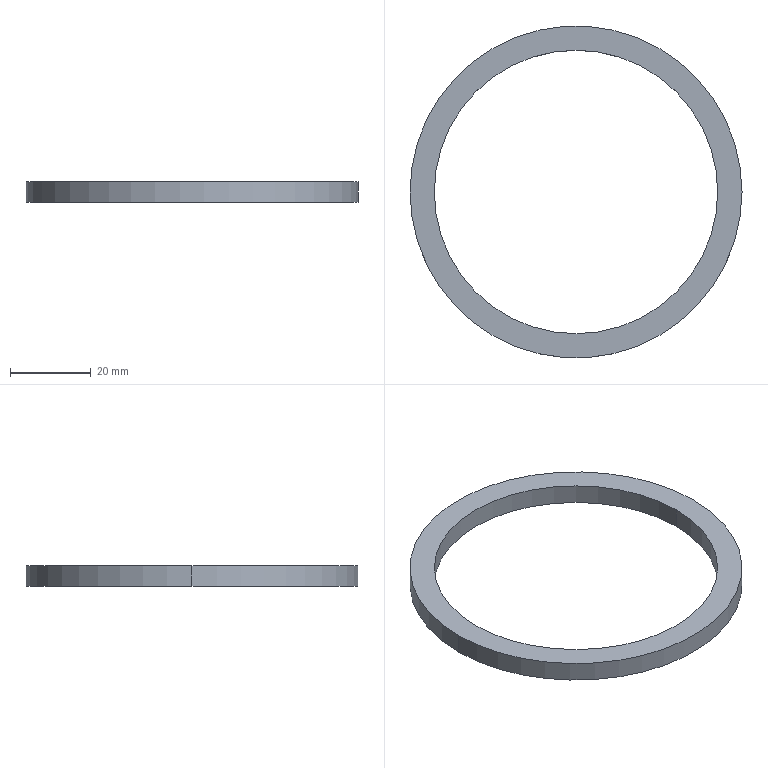Part | SolidWorks | features BaseBody 1 | 1 solid | 6 faces | box 82 x 82 x 5 mm | volume 7163 mm3 | cylinder 4 | plane 2 | commonest cylinder face diameters 70 x2 82 x2
STEP:
#1=CARTESIAN_POINT('',(-35.,0.,5.));
#2=VERTEX_POINT('',#1);
#3=CARTESIAN_POINT('',(35.,0.,5.));
#4=VERTEX_POINT('',#3);
#5=CARTESIAN_POINT('',(0.,0.,5.));
#6=DIRECTION('',(0.,0.,1.));
#7=DIRECTION('',(1.,0.,0.));
#8=AXIS2_PLACEMENT_3D('',#5,#6,#7);
#9=CIRCLE('',#8,35.);
#10=EDGE_CURVE('',#2,#4,#9,.T.);
#11=ORIENTED_EDGE('',*,*,#10,.T.);
#12=CARTESIAN_POINT('',(35.,0.,0.));
#13=VERTEX_POINT('',#12);
#14=CARTESIAN_POINT('',(35.,0.,5.));
#15=DIRECTION('',(0.,0.,-1.));
#16=VECTOR('',#15,1000.);
#17=LINE('',#14,#16);
#18=EDGE_CURVE('',#4,#13,#17,.T.);
#19=ORIENTED_EDGE('',*,*,#18,.T.);
#20=CARTESIAN_POINT('',(-35.,0.,0.));
#21=VERTEX_POINT('',#20);
#22=CARTESIAN_POINT('',(0.,0.,0.));
#23=DIRECTION('',(0.,0.,1.));
#24=DIRECTION('',(1.,0.,0.));
#25=AXIS2_PLACEMENT_3D('',#22,#23,#24);
#26=CIRCLE('',#25,35.);
#27=EDGE_CURVE('',#21,#13,#26,.T.);
#28=ORIENTED_EDGE('',*,*,#27,.F.);
#29=CARTESIAN_POINT('',(-35.,0.,5.));
#30=DIRECTION('',(0.,0.,-1.));
#31=VECTOR('',#30,1000.);
#32=LINE('',#29,#31);
#33=EDGE_CURVE('',#2,#21,#32,.T.);
#34=ORIENTED_EDGE('',*,*,#33,.F.);
#35=EDGE_LOOP('',(#11,#19,#28,#34));
#36=FACE_OUTER_BOUND('',#35,.T.);
#37=CARTESIAN_POINT('',(0.,0.,5.));
#38=DIRECTION('',(0.,0.,-1.));
#39=DIRECTION('',(-1.,0.,0.));
#40=AXIS2_PLACEMENT_3D('',#37,#38,#39);
#41=CYLINDRICAL_SURFACE('',#40,35.);
#42=ADVANCED_FACE('',(#36),#41,.F.);
#43=CARTESIAN_POINT('',(41.,0.,5.));
#44=VERTEX_POINT('',#43);
#45=CARTESIAN_POINT('',(-41.,0.,5.));
#46=VERTEX_POINT('',#45);
#47=CARTESIAN_POINT('',(0.,0.,5.));
#48=DIRECTION('',(0.,0.,1.));
#49=DIRECTION('',(1.,0.,0.));
#50=AXIS2_PLACEMENT_3D('',#47,#48,#49);
#51=CIRCLE('',#50,41.);
#52=EDGE_CURVE('',#44,#46,#51,.T.);
#53=ORIENTED_EDGE('',*,*,#52,.F.);
#54=CARTESIAN_POINT('',(41.,0.,0.));
#55=VERTEX_POINT('',#54);
#56=CARTESIAN_POINT('',(41.,0.,5.));
#57=DIRECTION('',(0.,0.,-1.));
#58=VECTOR('',#57,1000.);
#59=LINE('',#56,#58);
#60=EDGE_CURVE('',#44,#55,#59,.T.);
#61=ORIENTED_EDGE('',*,*,#60,.T.);
#62=CARTESIAN_POINT('',(-41.,0.,0.));
#63=VERTEX_POINT('',#62);
#64=CARTESIAN_POINT('',(0.,0.,0.));
#65=DIRECTION('',(0.,0.,1.));
#66=DIRECTION('',(1.,0.,0.));
#67=AXIS2_PLACEMENT_3D('',#64,#65,#66);
#68=CIRCLE('',#67,41.);
#69=EDGE_CURVE('',#55,#63,#68,.T.);
#70=ORIENTED_EDGE('',*,*,#69,.T.);
#71=CARTESIAN_POINT('',(-41.,0.,5.));
#72=DIRECTION('',(0.,0.,-1.));
#73=VECTOR('',#72,1000.);
#74=LINE('',#71,#73);
#75=EDGE_CURVE('',#46,#63,#74,.T.);
#76=ORIENTED_EDGE('',*,*,#75,.F.);
#77=EDGE_LOOP('',(#53,#61,#70,#76));
#78=FACE_OUTER_BOUND('',#77,.T.);
#79=CARTESIAN_POINT('',(0.,0.,5.));
#80=DIRECTION('',(0.,0.,-1.));
#81=DIRECTION('',(-1.,0.,0.));
#82=AXIS2_PLACEMENT_3D('',#79,#80,#81);
#83=CYLINDRICAL_SURFACE('',#82,41.);
#84=ADVANCED_FACE('',(#78),#83,.T.);
#85=ORIENTED_EDGE('',*,*,#10,.F.);
#86=CARTESIAN_POINT('',(0.,0.,5.));
#87=DIRECTION('',(0.,0.,1.));
#88=DIRECTION('',(1.,0.,0.));
#89=AXIS2_PLACEMENT_3D('',#86,#87,#88);
#90=CIRCLE('',#89,35.);
#91=EDGE_CURVE('',#4,#2,#90,.T.);
#92=ORIENTED_EDGE('',*,*,#91,.F.);
#93=EDGE_LOOP('',(#85,#92));
#94=FACE_BOUND('',#93,.T.);
#95=CARTESIAN_POINT('',(0.,0.,5.));
#96=DIRECTION('',(0.,0.,1.));
#97=DIRECTION('',(1.,0.,0.));
#98=AXIS2_PLACEMENT_3D('',#95,#96,#97);
#99=CIRCLE('',#98,41.);
#100=EDGE_CURVE('',#46,#44,#99,.T.);
#101=ORIENTED_EDGE('',*,*,#100,.T.);
#102=ORIENTED_EDGE('',*,*,#52,.T.);
#103=EDGE_LOOP('',(#101,#102));
#104=FACE_OUTER_BOUND('',#103,.T.);
#105=CARTESIAN_POINT('',(0.,0.,5.));
#106=DIRECTION('',(0.,0.,1.));
#107=DIRECTION('',(1.,0.,0.));
#108=AXIS2_PLACEMENT_3D('',#105,#106,#107);
#109=PLANE('',#108);
#110=ADVANCED_FACE('',(#94,#104),#109,.T.);
#111=ORIENTED_EDGE('',*,*,#27,.T.);
#112=CARTESIAN_POINT('',(0.,0.,0.));
#113=DIRECTION('',(0.,0.,1.));
#114=DIRECTION('',(1.,0.,0.));
#115=AXIS2_PLACEMENT_3D('',#112,#113,#114);
#116=CIRCLE('',#115,35.);
#117=EDGE_CURVE('',#13,#21,#116,.T.);
#118=ORIENTED_EDGE('',*,*,#117,.T.);
#119=EDGE_LOOP('',(#111,#118));
#120=FACE_BOUND('',#119,.T.);
#121=CARTESIAN_POINT('',(0.,0.,0.));
#122=DIRECTION('',(0.,0.,1.));
#123=DIRECTION('',(1.,0.,0.));
#124=AXIS2_PLACEMENT_3D('',#121,#122,#123);
#125=CIRCLE('',#124,41.);
#126=EDGE_CURVE('',#63,#55,#125,.T.);
#127=ORIENTED_EDGE('',*,*,#126,.F.);
#128=ORIENTED_EDGE('',*,*,#69,.F.);
#129=EDGE_LOOP('',(#127,#128));
#130=FACE_OUTER_BOUND('',#129,.T.);
#131=CARTESIAN_POINT('',(0.,0.,0.));
#132=DIRECTION('',(0.,0.,1.));
#133=DIRECTION('',(1.,0.,0.));
#134=AXIS2_PLACEMENT_3D('',#131,#132,#133);
#135=PLANE('',#134);
#136=ADVANCED_FACE('',(#120,#130),#135,.F.);
#137=ORIENTED_EDGE('',*,*,#60,.F.);
#138=ORIENTED_EDGE('',*,*,#100,.F.);
#139=ORIENTED_EDGE('',*,*,#75,.T.);
#140=ORIENTED_EDGE('',*,*,#126,.T.);
#141=EDGE_LOOP('',(#137,#138,#139,#140));
#142=FACE_OUTER_BOUND('',#141,.T.);
#143=CARTESIAN_POINT('',(0.,0.,5.));
#144=DIRECTION('',(0.,0.,-1.));
#145=DIRECTION('',(-1.,0.,0.));
#146=AXIS2_PLACEMENT_3D('',#143,#144,#145);
#147=CYLINDRICAL_SURFACE('',#146,41.);
#148=ADVANCED_FACE('',(#142),#147,.T.);
#149=ORIENTED_EDGE('',*,*,#18,.F.);
#150=ORIENTED_EDGE('',*,*,#91,.T.);
#151=ORIENTED_EDGE('',*,*,#33,.T.);
#152=ORIENTED_EDGE('',*,*,#117,.F.);
#153=EDGE_LOOP('',(#149,#150,#151,#152));
#154=FACE_OUTER_BOUND('',#153,.T.);
#155=CARTESIAN_POINT('',(0.,0.,5.));
#156=DIRECTION('',(0.,0.,-1.));
#157=DIRECTION('',(-1.,0.,0.));
#158=AXIS2_PLACEMENT_3D('',#155,#156,#157);
#159=CYLINDRICAL_SURFACE('',#158,35.);
#160=ADVANCED_FACE('',(#154),#159,.F.);
#161=CLOSED_SHELL('',(#42,#84,#110,#136,#148,#160));
#162=MANIFOLD_SOLID_BREP('',#161);
#163=CARTESIAN_POINT('',(0.,0.,0.));
#164=DIRECTION('',(0.,0.,1.));
#165=DIRECTION('',(1.,0.,0.));
#166=AXIS2_PLACEMENT_3D('',#163,#164,#165);
#167=(LENGTH_UNIT()NAMED_UNIT(*)SI_UNIT(.MILLI.,.METRE.));
#168=UNCERTAINTY_MEASURE_WITH_UNIT(LENGTH_MEASURE(0.00001),#167,'','');
#169=(NAMED_UNIT(*)PLANE_ANGLE_UNIT()SI_UNIT($,.RADIAN.));
#170=(NAMED_UNIT(*)SI_UNIT($,.STERADIAN.)SOLID_ANGLE_UNIT());
#171=(GEOMETRIC_REPRESENTATION_CONTEXT(3)GLOBAL_UNCERTAINTY_ASSIGNED_CONTEXT((#168))GLOBAL_UNIT_ASSIGNED_CONTEXT((#167,#169,#170))REPRESENTATION_CONTEXT('',''));
#172=ADVANCED_BREP_SHAPE_REPRESENTATION('',(#162,#166),#171);